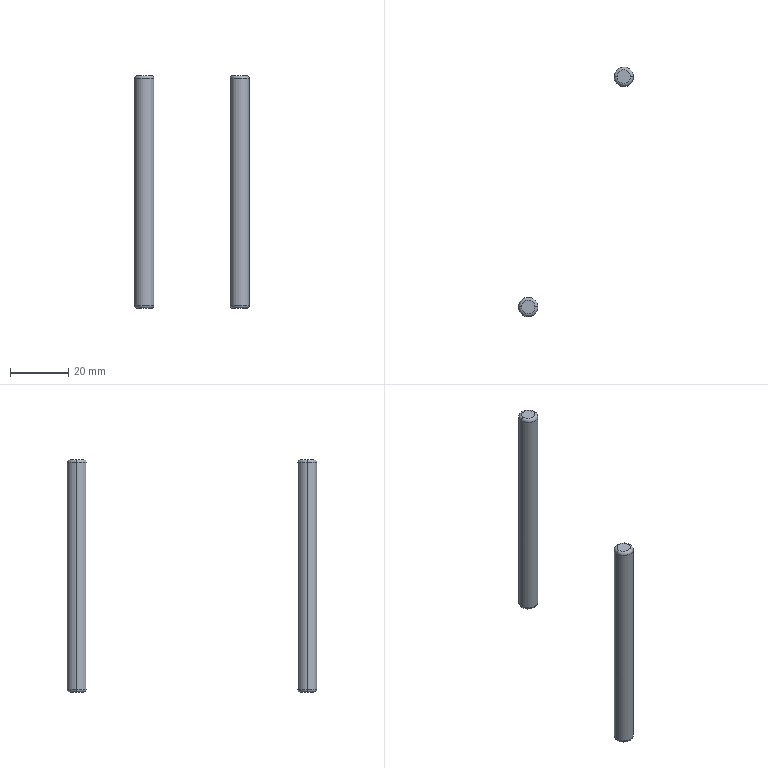Part | SolidWorks | features Fillet 2, Extrusion 1 | 2 solids | 16 faces | box 39.358 x 85.684 x 80 mm | volume 5457 mm3 | torus 8 | cylinder 4 | plane 4 | commonest cylinder face diameters 6.6 x4
STEP:
#1=CARTESIAN_POINT('',(-18.679,-39.542,0.));
#2=VERTEX_POINT('',#1);
#3=CARTESIAN_POINT('',(-14.079,-39.542,0.));
#4=VERTEX_POINT('',#3);
#5=CARTESIAN_POINT('',(-16.379,-39.542,0.));
#6=DIRECTION('',(0.,0.,-1.));
#7=DIRECTION('',(1.,0.,0.));
#8=AXIS2_PLACEMENT_3D('',#5,#6,#7);
#9=CIRCLE('',#8,2.3);
#10=EDGE_CURVE('',#2,#4,#9,.T.);
#11=ORIENTED_EDGE('',*,*,#10,.F.);
#12=CARTESIAN_POINT('',(-19.679,-39.542,1.));
#13=VERTEX_POINT('',#12);
#14=CARTESIAN_POINT('',(-18.679,-39.542,1.));
#15=DIRECTION('',(0.,1.,0.));
#16=DIRECTION('',(-1.,0.,0.));
#17=AXIS2_PLACEMENT_3D('',#14,#15,#16);
#18=CIRCLE('',#17,1.);
#19=EDGE_CURVE('',#2,#13,#18,.T.);
#20=ORIENTED_EDGE('',*,*,#19,.T.);
#21=CARTESIAN_POINT('',(-13.079,-39.542,1.));
#22=VERTEX_POINT('',#21);
#23=CARTESIAN_POINT('',(-16.379,-39.542,1.));
#24=DIRECTION('',(0.,0.,1.));
#25=DIRECTION('',(1.,0.,0.));
#26=AXIS2_PLACEMENT_3D('',#23,#24,#25);
#27=CIRCLE('',#26,3.3);
#28=EDGE_CURVE('',#22,#13,#27,.T.);
#29=ORIENTED_EDGE('',*,*,#28,.F.);
#30=CARTESIAN_POINT('',(-14.079,-39.542,1.));
#31=DIRECTION('',(0.,-1.,0.));
#32=DIRECTION('',(0.,0.,-1.));
#33=AXIS2_PLACEMENT_3D('',#30,#31,#32);
#34=CIRCLE('',#33,1.);
#35=EDGE_CURVE('',#4,#22,#34,.T.);
#36=ORIENTED_EDGE('',*,*,#35,.F.);
#37=EDGE_LOOP('',(#11,#20,#29,#36));
#38=FACE_OUTER_BOUND('',#37,.T.);
#39=CARTESIAN_POINT('',(-16.379,-39.542,1.));
#40=DIRECTION('',(0.,0.,1.));
#41=DIRECTION('',(1.,0.,0.));
#42=AXIS2_PLACEMENT_3D('',#39,#40,#41);
#43=TOROIDAL_SURFACE('',#42,2.3,1.);
#44=ADVANCED_FACE('',(#38),#43,.T.);
#45=CARTESIAN_POINT('',(-19.679,-39.542,79.));
#46=VERTEX_POINT('',#45);
#47=CARTESIAN_POINT('',(-13.079,-39.542,79.));
#48=VERTEX_POINT('',#47);
#49=CARTESIAN_POINT('',(-16.379,-39.542,79.));
#50=DIRECTION('',(0.,0.,-1.));
#51=DIRECTION('',(1.,0.,0.));
#52=AXIS2_PLACEMENT_3D('',#49,#50,#51);
#53=CIRCLE('',#52,3.3);
#54=EDGE_CURVE('',#46,#48,#53,.T.);
#55=ORIENTED_EDGE('',*,*,#54,.F.);
#56=CARTESIAN_POINT('',(-18.679,-39.542,80.));
#57=VERTEX_POINT('',#56);
#58=CARTESIAN_POINT('',(-18.679,-39.542,79.));
#59=DIRECTION('',(0.,1.,0.));
#60=DIRECTION('',(-1.,0.,0.));
#61=AXIS2_PLACEMENT_3D('',#58,#59,#60);
#62=CIRCLE('',#61,1.);
#63=EDGE_CURVE('',#46,#57,#62,.T.);
#64=ORIENTED_EDGE('',*,*,#63,.T.);
#65=CARTESIAN_POINT('',(-14.079,-39.542,80.));
#66=VERTEX_POINT('',#65);
#67=CARTESIAN_POINT('',(-16.379,-39.542,80.));
#68=DIRECTION('',(0.,0.,1.));
#69=DIRECTION('',(1.,0.,0.));
#70=AXIS2_PLACEMENT_3D('',#67,#68,#69);
#71=CIRCLE('',#70,2.3);
#72=EDGE_CURVE('',#66,#57,#71,.T.);
#73=ORIENTED_EDGE('',*,*,#72,.F.);
#74=CARTESIAN_POINT('',(-14.079,-39.542,79.));
#75=DIRECTION('',(0.,-1.,0.));
#76=DIRECTION('',(0.,0.,-1.));
#77=AXIS2_PLACEMENT_3D('',#74,#75,#76);
#78=CIRCLE('',#77,1.);
#79=EDGE_CURVE('',#48,#66,#78,.T.);
#80=ORIENTED_EDGE('',*,*,#79,.F.);
#81=EDGE_LOOP('',(#55,#64,#73,#80));
#82=FACE_OUTER_BOUND('',#81,.T.);
#83=CARTESIAN_POINT('',(-16.379,-39.542,79.));
#84=DIRECTION('',(0.,0.,1.));
#85=DIRECTION('',(1.,0.,0.));
#86=AXIS2_PLACEMENT_3D('',#83,#84,#85);
#87=TOROIDAL_SURFACE('',#86,2.3,1.);
#88=ADVANCED_FACE('',(#82),#87,.T.);
#89=ORIENTED_EDGE('',*,*,#54,.T.);
#90=CARTESIAN_POINT('',(-13.079,-39.542,80.));
#91=DIRECTION('',(0.,0.,-1.));
#92=VECTOR('',#91,1000.);
#93=LINE('',#90,#92);
#94=EDGE_CURVE('',#48,#22,#93,.T.);
#95=ORIENTED_EDGE('',*,*,#94,.T.);
#96=ORIENTED_EDGE('',*,*,#28,.T.);
#97=CARTESIAN_POINT('',(-19.679,-39.542,80.));
#98=DIRECTION('',(0.,0.,-1.));
#99=VECTOR('',#98,1000.);
#100=LINE('',#97,#99);
#101=EDGE_CURVE('',#46,#13,#100,.T.);
#102=ORIENTED_EDGE('',*,*,#101,.F.);
#103=EDGE_LOOP('',(#89,#95,#96,#102));
#104=FACE_OUTER_BOUND('',#103,.T.);
#105=CARTESIAN_POINT('',(-16.379,-39.542,80.));
#106=DIRECTION('',(0.,0.,-1.));
#107=DIRECTION('',(-1.,0.,0.));
#108=AXIS2_PLACEMENT_3D('',#105,#106,#107);
#109=CYLINDRICAL_SURFACE('',#108,3.3);
#110=ADVANCED_FACE('',(#104),#109,.T.);
#111=ORIENTED_EDGE('',*,*,#94,.F.);
#112=CARTESIAN_POINT('',(-16.379,-39.542,79.));
#113=DIRECTION('',(0.,0.,-1.));
#114=DIRECTION('',(1.,0.,0.));
#115=AXIS2_PLACEMENT_3D('',#112,#113,#114);
#116=CIRCLE('',#115,3.3);
#117=EDGE_CURVE('',#48,#46,#116,.T.);
#118=ORIENTED_EDGE('',*,*,#117,.T.);
#119=ORIENTED_EDGE('',*,*,#101,.T.);
#120=CARTESIAN_POINT('',(-16.379,-39.542,1.));
#121=DIRECTION('',(0.,0.,1.));
#122=DIRECTION('',(1.,0.,0.));
#123=AXIS2_PLACEMENT_3D('',#120,#121,#122);
#124=CIRCLE('',#123,3.3);
#125=EDGE_CURVE('',#13,#22,#124,.T.);
#126=ORIENTED_EDGE('',*,*,#125,.T.);
#127=EDGE_LOOP('',(#111,#118,#119,#126));
#128=FACE_OUTER_BOUND('',#127,.T.);
#129=CARTESIAN_POINT('',(-16.379,-39.542,80.));
#130=DIRECTION('',(0.,0.,-1.));
#131=DIRECTION('',(-1.,0.,0.));
#132=AXIS2_PLACEMENT_3D('',#129,#130,#131);
#133=CYLINDRICAL_SURFACE('',#132,3.3);
#134=ADVANCED_FACE('',(#128),#133,.T.);
#135=ORIENTED_EDGE('',*,*,#72,.T.);
#136=CARTESIAN_POINT('',(-16.379,-39.542,80.));
#137=DIRECTION('',(0.,0.,1.));
#138=DIRECTION('',(1.,0.,0.));
#139=AXIS2_PLACEMENT_3D('',#136,#137,#138);
#140=CIRCLE('',#139,2.3);
#141=EDGE_CURVE('',#57,#66,#140,.T.);
#142=ORIENTED_EDGE('',*,*,#141,.T.);
#143=EDGE_LOOP('',(#135,#142));
#144=FACE_OUTER_BOUND('',#143,.T.);
#145=CARTESIAN_POINT('',(-16.379,-39.542,80.));
#146=DIRECTION('',(0.,0.,1.));
#147=DIRECTION('',(1.,0.,0.));
#148=AXIS2_PLACEMENT_3D('',#145,#146,#147);
#149=PLANE('',#148);
#150=ADVANCED_FACE('',(#144),#149,.T.);
#151=CARTESIAN_POINT('',(-16.379,-39.542,0.));
#152=DIRECTION('',(0.,0.,-1.));
#153=DIRECTION('',(1.,0.,0.));
#154=AXIS2_PLACEMENT_3D('',#151,#152,#153);
#155=CIRCLE('',#154,2.3);
#156=EDGE_CURVE('',#4,#2,#155,.T.);
#157=ORIENTED_EDGE('',*,*,#156,.T.);
#158=ORIENTED_EDGE('',*,*,#10,.T.);
#159=EDGE_LOOP('',(#157,#158));
#160=FACE_OUTER_BOUND('',#159,.T.);
#161=CARTESIAN_POINT('',(-16.379,-39.542,0.));
#162=DIRECTION('',(0.,0.,1.));
#163=DIRECTION('',(1.,0.,0.));
#164=AXIS2_PLACEMENT_3D('',#161,#162,#163);
#165=PLANE('',#164);
#166=ADVANCED_FACE('',(#160),#165,.F.);
#167=ORIENTED_EDGE('',*,*,#63,.F.);
#168=ORIENTED_EDGE('',*,*,#117,.F.);
#169=ORIENTED_EDGE('',*,*,#79,.T.);
#170=ORIENTED_EDGE('',*,*,#141,.F.);
#171=EDGE_LOOP('',(#167,#168,#169,#170));
#172=FACE_OUTER_BOUND('',#171,.T.);
#173=CARTESIAN_POINT('',(-16.379,-39.542,79.));
#174=DIRECTION('',(0.,0.,1.));
#175=DIRECTION('',(1.,0.,0.));
#176=AXIS2_PLACEMENT_3D('',#173,#174,#175);
#177=TOROIDAL_SURFACE('',#176,2.3,1.);
#178=ADVANCED_FACE('',(#172),#177,.T.);
#179=ORIENTED_EDGE('',*,*,#19,.F.);
#180=ORIENTED_EDGE('',*,*,#156,.F.);
#181=ORIENTED_EDGE('',*,*,#35,.T.);
#182=ORIENTED_EDGE('',*,*,#125,.F.);
#183=EDGE_LOOP('',(#179,#180,#181,#182));
#184=FACE_OUTER_BOUND('',#183,.T.);
#185=CARTESIAN_POINT('',(-16.379,-39.542,1.));
#186=DIRECTION('',(0.,0.,1.));
#187=DIRECTION('',(1.,0.,0.));
#188=AXIS2_PLACEMENT_3D('',#185,#186,#187);
#189=TOROIDAL_SURFACE('',#188,2.3,1.);
#190=ADVANCED_FACE('',(#184),#189,.T.);
#191=CLOSED_SHELL('',(#44,#88,#110,#134,#150,#166,#178,#190));
#192=MANIFOLD_SOLID_BREP('',#191);
#193=CARTESIAN_POINT('',(14.079,39.542,0.));
#194=VERTEX_POINT('',#193);
#195=CARTESIAN_POINT('',(18.679,39.542,0.));
#196=VERTEX_POINT('',#195);
#197=CARTESIAN_POINT('',(16.379,39.542,0.));
#198=DIRECTION('',(0.,0.,-1.));
#199=DIRECTION('',(1.,0.,0.));
#200=AXIS2_PLACEMENT_3D('',#197,#198,#199);
#201=CIRCLE('',#200,2.3);
#202=EDGE_CURVE('',#194,#196,#201,.T.);
#203=ORIENTED_EDGE('',*,*,#202,.F.);
#204=CARTESIAN_POINT('',(13.079,39.542,1.));
#205=VERTEX_POINT('',#204);
#206=CARTESIAN_POINT('',(14.079,39.542,1.));
#207=DIRECTION('',(0.,1.,0.));
#208=DIRECTION('',(-1.,0.,0.));
#209=AXIS2_PLACEMENT_3D('',#206,#207,#208);
#210=CIRCLE('',#209,1.);
#211=EDGE_CURVE('',#194,#205,#210,.T.);
#212=ORIENTED_EDGE('',*,*,#211,.T.);
#213=CARTESIAN_POINT('',(19.679,39.542,1.));
#214=VERTEX_POINT('',#213);
#215=CARTESIAN_POINT('',(16.379,39.542,1.));
#216=DIRECTION('',(0.,0.,1.));
#217=DIRECTION('',(1.,0.,0.));
#218=AXIS2_PLACEMENT_3D('',#215,#216,#217);
#219=CIRCLE('',#218,3.3);
#220=EDGE_CURVE('',#214,#205,#219,.T.);
#221=ORIENTED_EDGE('',*,*,#220,.F.);
#222=CARTESIAN_POINT('',(18.679,39.542,1.));
#223=DIRECTION('',(0.,-1.,0.));
#224=DIRECTION('',(0.,0.,-1.));
#225=AXIS2_PLACEMENT_3D('',#222,#223,#224);
#226=CIRCLE('',#225,1.);
#227=EDGE_CURVE('',#196,#214,#226,.T.);
#228=ORIENTED_EDGE('',*,*,#227,.F.);
#229=EDGE_LOOP('',(#203,#212,#221,#228));
#230=FACE_OUTER_BOUND('',#229,.T.);
#231=CARTESIAN_POINT('',(16.379,39.542,1.));
#232=DIRECTION('',(0.,0.,1.));
#233=DIRECTION('',(1.,0.,0.));
#234=AXIS2_PLACEMENT_3D('',#231,#232,#233);
#235=TOROIDAL_SURFACE('',#234,2.3,1.);
#236=ADVANCED_FACE('',(#230),#235,.T.);
#237=CARTESIAN_POINT('',(13.079,39.542,79.));
#238=VERTEX_POINT('',#237);
#239=CARTESIAN_POINT('',(19.679,39.542,79.));
#240=VERTEX_POINT('',#239);
#241=CARTESIAN_POINT('',(16.379,39.542,79.));
#242=DIRECTION('',(0.,0.,-1.));
#243=DIRECTION('',(1.,0.,0.));
#244=AXIS2_PLACEMENT_3D('',#241,#242,#243);
#245=CIRCLE('',#244,3.3);
#246=EDGE_CURVE('',#238,#240,#245,.T.);
#247=ORIENTED_EDGE('',*,*,#246,.F.);
#248=CARTESIAN_POINT('',(14.079,39.542,80.));
#249=VERTEX_POINT('',#248);
#250=CARTESIAN_POINT('',(14.079,39.542,79.));
#251=DIRECTION('',(0.,1.,0.));
#252=DIRECTION('',(-1.,0.,0.));
#253=AXIS2_PLACEMENT_3D('',#250,#251,#252);
#254=CIRCLE('',#253,1.);
#255=EDGE_CURVE('',#238,#249,#254,.T.);
#256=ORIENTED_EDGE('',*,*,#255,.T.);
#257=CARTESIAN_POINT('',(18.679,39.542,80.));
#258=VERTEX_POINT('',#257);
#259=CARTESIAN_POINT('',(16.379,39.542,80.));
#260=DIRECTION('',(0.,0.,1.));
#261=DIRECTION('',(1.,0.,0.));
#262=AXIS2_PLACEMENT_3D('',#259,#260,#261);
#263=CIRCLE('',#262,2.3);
#264=EDGE_CURVE('',#258,#249,#263,.T.);
#265=ORIENTED_EDGE('',*,*,#264,.F.);
#266=CARTESIAN_POINT('',(18.679,39.542,79.));
#267=DIRECTION('',(0.,-1.,0.));
#268=DIRECTION('',(0.,0.,-1.));
#269=AXIS2_PLACEMENT_3D('',#266,#267,#268);
#270=CIRCLE('',#269,1.);
#271=EDGE_CURVE('',#240,#258,#270,.T.);
#272=ORIENTED_EDGE('',*,*,#271,.F.);
#273=EDGE_LOOP('',(#247,#256,#265,#272));
#274=FACE_OUTER_BOUND('',#273,.T.);
#275=CARTESIAN_POINT('',(16.379,39.542,79.));
#276=DIRECTION('',(0.,0.,1.));
#277=DIRECTION('',(1.,0.,0.));
#278=AXIS2_PLACEMENT_3D('',#275,#276,#277);
#279=TOROIDAL_SURFACE('',#278,2.3,1.);
#280=ADVANCED_FACE('',(#274),#279,.T.);
#281=ORIENTED_EDGE('',*,*,#246,.T.);
#282=CARTESIAN_POINT('',(19.679,39.542,80.));
#283=DIRECTION('',(0.,0.,-1.));
#284=VECTOR('',#283,1000.);
#285=LINE('',#282,#284);
#286=EDGE_CURVE('',#240,#214,#285,.T.);
#287=ORIENTED_EDGE('',*,*,#286,.T.);
#288=ORIENTED_EDGE('',*,*,#220,.T.);
#289=CARTESIAN_POINT('',(13.079,39.542,80.));
#290=DIRECTION('',(0.,0.,-1.));
#291=VECTOR('',#290,1000.);
#292=LINE('',#289,#291);
#293=EDGE_CURVE('',#238,#205,#292,.T.);
#294=ORIENTED_EDGE('',*,*,#293,.F.);
#295=EDGE_LOOP('',(#281,#287,#288,#294));
#296=FACE_OUTER_BOUND('',#295,.T.);
#297=CARTESIAN_POINT('',(16.379,39.542,80.));
#298=DIRECTION('',(0.,0.,-1.));
#299=DIRECTION('',(-1.,0.,0.));
#300=AXIS2_PLACEMENT_3D('',#297,#298,#299);
#301=CYLINDRICAL_SURFACE('',#300,3.3);
#302=ADVANCED_FACE('',(#296),#301,.T.);
#303=ORIENTED_EDGE('',*,*,#286,.F.);
#304=CARTESIAN_POINT('',(16.379,39.542,79.));
#305=DIRECTION('',(0.,0.,-1.));
#306=DIRECTION('',(1.,0.,0.));
#307=AXIS2_PLACEMENT_3D('',#304,#305,#306);
#308=CIRCLE('',#307,3.3);
#309=EDGE_CURVE('',#240,#238,#308,.T.);
#310=ORIENTED_EDGE('',*,*,#309,.T.);
#311=ORIENTED_EDGE('',*,*,#293,.T.);
#312=CARTESIAN_POINT('',(16.379,39.542,1.));
#313=DIRECTION('',(0.,0.,1.));
#314=DIRECTION('',(1.,0.,0.));
#315=AXIS2_PLACEMENT_3D('',#312,#313,#314);
#316=CIRCLE('',#315,3.3);
#317=EDGE_CURVE('',#205,#214,#316,.T.);
#318=ORIENTED_EDGE('',*,*,#317,.T.);
#319=EDGE_LOOP('',(#303,#310,#311,#318));
#320=FACE_OUTER_BOUND('',#319,.T.);
#321=CARTESIAN_POINT('',(16.379,39.542,80.));
#322=DIRECTION('',(0.,0.,-1.));
#323=DIRECTION('',(-1.,0.,0.));
#324=AXIS2_PLACEMENT_3D('',#321,#322,#323);
#325=CYLINDRICAL_SURFACE('',#324,3.3);
#326=ADVANCED_FACE('',(#320),#325,.T.);
#327=ORIENTED_EDGE('',*,*,#264,.T.);
#328=CARTESIAN_POINT('',(16.379,39.542,80.));
#329=DIRECTION('',(0.,0.,1.));
#330=DIRECTION('',(1.,0.,0.));
#331=AXIS2_PLACEMENT_3D('',#328,#329,#330);
#332=CIRCLE('',#331,2.3);
#333=EDGE_CURVE('',#249,#258,#332,.T.);
#334=ORIENTED_EDGE('',*,*,#333,.T.);
#335=EDGE_LOOP('',(#327,#334));
#336=FACE_OUTER_BOUND('',#335,.T.);
#337=CARTESIAN_POINT('',(16.379,39.542,80.));
#338=DIRECTION('',(0.,0.,1.));
#339=DIRECTION('',(1.,0.,0.));
#340=AXIS2_PLACEMENT_3D('',#337,#338,#339);
#341=PLANE('',#340);
#342=ADVANCED_FACE('',(#336),#341,.T.);
#343=CARTESIAN_POINT('',(16.379,39.542,0.));
#344=DIRECTION('',(0.,0.,-1.));
#345=DIRECTION('',(1.,0.,0.));
#346=AXIS2_PLACEMENT_3D('',#343,#344,#345);
#347=CIRCLE('',#346,2.3);
#348=EDGE_CURVE('',#196,#194,#347,.T.);
#349=ORIENTED_EDGE('',*,*,#348,.T.);
#350=ORIENTED_EDGE('',*,*,#202,.T.);
#351=EDGE_LOOP('',(#349,#350));
#352=FACE_OUTER_BOUND('',#351,.T.);
#353=CARTESIAN_POINT('',(16.379,39.542,0.));
#354=DIRECTION('',(0.,0.,1.));
#355=DIRECTION('',(1.,0.,0.));
#356=AXIS2_PLACEMENT_3D('',#353,#354,#355);
#357=PLANE('',#356);
#358=ADVANCED_FACE('',(#352),#357,.F.);
#359=ORIENTED_EDGE('',*,*,#255,.F.);
#360=ORIENTED_EDGE('',*,*,#309,.F.);
#361=ORIENTED_EDGE('',*,*,#271,.T.);
#362=ORIENTED_EDGE('',*,*,#333,.F.);
#363=EDGE_LOOP('',(#359,#360,#361,#362));
#364=FACE_OUTER_BOUND('',#363,.T.);
#365=CARTESIAN_POINT('',(16.379,39.542,79.));
#366=DIRECTION('',(0.,0.,1.));
#367=DIRECTION('',(1.,0.,0.));
#368=AXIS2_PLACEMENT_3D('',#365,#366,#367);
#369=TOROIDAL_SURFACE('',#368,2.3,1.);
#370=ADVANCED_FACE('',(#364),#369,.T.);
#371=ORIENTED_EDGE('',*,*,#211,.F.);
#372=ORIENTED_EDGE('',*,*,#348,.F.);
#373=ORIENTED_EDGE('',*,*,#227,.T.);
#374=ORIENTED_EDGE('',*,*,#317,.F.);
#375=EDGE_LOOP('',(#371,#372,#373,#374));
#376=FACE_OUTER_BOUND('',#375,.T.);
#377=CARTESIAN_POINT('',(16.379,39.542,1.));
#378=DIRECTION('',(0.,0.,1.));
#379=DIRECTION('',(1.,0.,0.));
#380=AXIS2_PLACEMENT_3D('',#377,#378,#379);
#381=TOROIDAL_SURFACE('',#380,2.3,1.);
#382=ADVANCED_FACE('',(#376),#381,.T.);
#383=CLOSED_SHELL('',(#236,#280,#302,#326,#342,#358,#370,#382));
#384=MANIFOLD_SOLID_BREP('',#383);
#385=CARTESIAN_POINT('',(0.,0.,0.));
#386=DIRECTION('',(0.,0.,1.));
#387=DIRECTION('',(1.,0.,0.));
#388=AXIS2_PLACEMENT_3D('',#385,#386,#387);
#389=(LENGTH_UNIT()NAMED_UNIT(*)SI_UNIT(.MILLI.,.METRE.));
#390=UNCERTAINTY_MEASURE_WITH_UNIT(LENGTH_MEASURE(0.00001),#389,'','');
#391=(NAMED_UNIT(*)PLANE_ANGLE_UNIT()SI_UNIT($,.RADIAN.));
#392=(NAMED_UNIT(*)SI_UNIT($,.STERADIAN.)SOLID_ANGLE_UNIT());
#393=(GEOMETRIC_REPRESENTATION_CONTEXT(3)GLOBAL_UNCERTAINTY_ASSIGNED_CONTEXT((#390))GLOBAL_UNIT_ASSIGNED_CONTEXT((#389,#391,#392))REPRESENTATION_CONTEXT('',''));
#394=ADVANCED_BREP_SHAPE_REPRESENTATION('',(#192,#384,#388),#393);